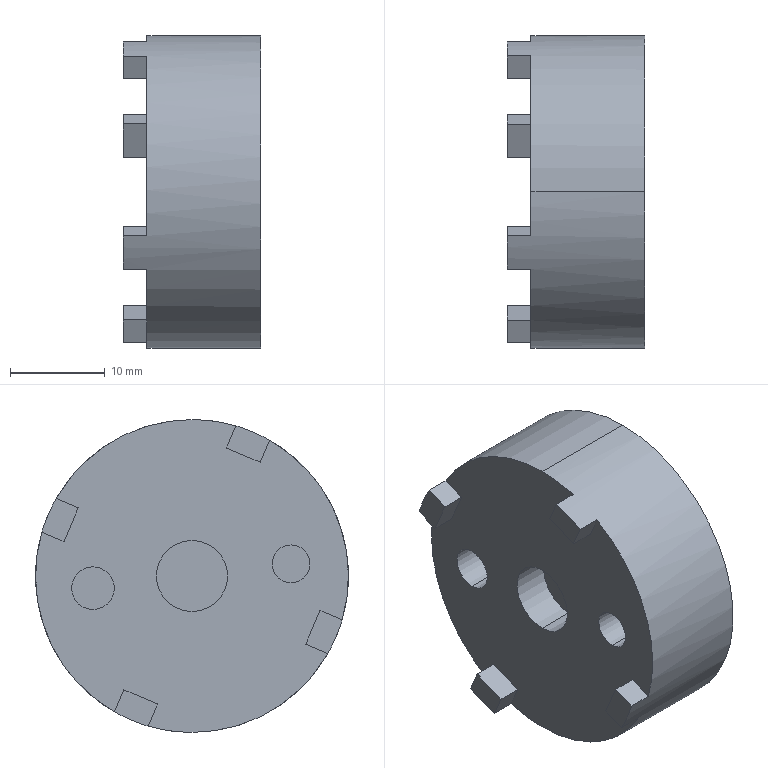Part | SolidWorks | features Cut 2, ICE 2, CirPattern 1, Extrusion 1 | 1 solid | 34 faces | box 14.5 x 33 x 33 mm | volume 10024 mm3 | plane 26 | cylinder 8 | commonest cylinder face diameters 4 x2 4.5 x2 7.5 x2 33 x2
STEP:
#1=CARTESIAN_POINT('',(4.,-10.447,3.283));
#2=VERTEX_POINT('',#1);
#3=CARTESIAN_POINT('',(4.,-10.447,-0.7173));
#4=VERTEX_POINT('',#3);
#5=CARTESIAN_POINT('',(4.,-10.447,1.283));
#6=DIRECTION('',(1.,0.,0.));
#7=DIRECTION('',(0.,0.,1.));
#8=AXIS2_PLACEMENT_3D('',#5,#6,#7);
#9=CIRCLE('',#8,2.);
#10=EDGE_CURVE('',#2,#4,#9,.T.);
#11=ORIENTED_EDGE('',*,*,#10,.T.);
#12=CARTESIAN_POINT('',(0.,-10.447,-0.7173));
#13=VERTEX_POINT('',#12);
#14=CARTESIAN_POINT('',(10.364,-10.447,-0.7173));
#15=DIRECTION('',(-1.,0.,0.));
#16=VECTOR('',#15,1000.);
#17=LINE('',#14,#16);
#18=EDGE_CURVE('',#4,#13,#17,.T.);
#19=ORIENTED_EDGE('',*,*,#18,.T.);
#20=CARTESIAN_POINT('',(0.,-10.447,3.283));
#21=VERTEX_POINT('',#20);
#22=CARTESIAN_POINT('',(0.,-10.447,1.283));
#23=DIRECTION('',(-1.,0.,0.));
#24=DIRECTION('',(0.,0.,1.));
#25=AXIS2_PLACEMENT_3D('',#22,#23,#24);
#26=CIRCLE('',#25,2.);
#27=EDGE_CURVE('',#13,#21,#26,.T.);
#28=ORIENTED_EDGE('',*,*,#27,.T.);
#29=CARTESIAN_POINT('',(10.364,-10.447,3.283));
#30=DIRECTION('',(-1.,0.,0.));
#31=VECTOR('',#30,1000.);
#32=LINE('',#29,#31);
#33=EDGE_CURVE('',#2,#21,#32,.T.);
#34=ORIENTED_EDGE('',*,*,#33,.F.);
#35=EDGE_LOOP('',(#11,#19,#28,#34));
#36=FACE_OUTER_BOUND('',#35,.T.);
#37=CARTESIAN_POINT('',(10.364,-10.447,1.283));
#38=DIRECTION('',(-1.,0.,0.));
#39=DIRECTION('',(0.,0.,1.));
#40=AXIS2_PLACEMENT_3D('',#37,#38,#39);
#41=CYLINDRICAL_SURFACE('',#40,2.);
#42=ADVANCED_FACE('',(#36),#41,.F.);
#43=CARTESIAN_POINT('',(4.,10.447,0.9673));
#44=VERTEX_POINT('',#43);
#45=CARTESIAN_POINT('',(4.,10.447,-3.533));
#46=VERTEX_POINT('',#45);
#47=CARTESIAN_POINT('',(4.,10.447,-1.283));
#48=DIRECTION('',(1.,0.,0.));
#49=DIRECTION('',(0.,0.,1.));
#50=AXIS2_PLACEMENT_3D('',#47,#48,#49);
#51=CIRCLE('',#50,2.25);
#52=EDGE_CURVE('',#44,#46,#51,.T.);
#53=ORIENTED_EDGE('',*,*,#52,.T.);
#54=CARTESIAN_POINT('',(0.,10.447,-3.533));
#55=VERTEX_POINT('',#54);
#56=CARTESIAN_POINT('',(10.364,10.447,-3.533));
#57=DIRECTION('',(-1.,0.,0.));
#58=VECTOR('',#57,1000.);
#59=LINE('',#56,#58);
#60=EDGE_CURVE('',#46,#55,#59,.T.);
#61=ORIENTED_EDGE('',*,*,#60,.T.);
#62=CARTESIAN_POINT('',(0.,10.447,0.9673));
#63=VERTEX_POINT('',#62);
#64=CARTESIAN_POINT('',(0.,10.447,-1.283));
#65=DIRECTION('',(-1.,0.,0.));
#66=DIRECTION('',(0.,0.,1.));
#67=AXIS2_PLACEMENT_3D('',#64,#65,#66);
#68=CIRCLE('',#67,2.25);
#69=EDGE_CURVE('',#55,#63,#68,.T.);
#70=ORIENTED_EDGE('',*,*,#69,.T.);
#71=CARTESIAN_POINT('',(10.364,10.447,0.9673));
#72=DIRECTION('',(-1.,0.,0.));
#73=VECTOR('',#72,1000.);
#74=LINE('',#71,#73);
#75=EDGE_CURVE('',#44,#63,#74,.T.);
#76=ORIENTED_EDGE('',*,*,#75,.F.);
#77=EDGE_LOOP('',(#53,#61,#70,#76));
#78=FACE_OUTER_BOUND('',#77,.T.);
#79=CARTESIAN_POINT('',(10.364,10.447,-1.283));
#80=DIRECTION('',(-1.,0.,0.));
#81=DIRECTION('',(0.,0.,1.));
#82=AXIS2_PLACEMENT_3D('',#79,#80,#81);
#83=CYLINDRICAL_SURFACE('',#82,2.25);
#84=ADVANCED_FACE('',(#78),#83,.F.);
#85=CARTESIAN_POINT('',(4.,0.,-3.75));
#86=VERTEX_POINT('',#85);
#87=CARTESIAN_POINT('',(4.,0.,3.75));
#88=VERTEX_POINT('',#87);
#89=CARTESIAN_POINT('',(4.,0.,0.));
#90=DIRECTION('',(-1.,0.,0.));
#91=DIRECTION('',(0.,0.,1.));
#92=AXIS2_PLACEMENT_3D('',#89,#90,#91);
#93=CIRCLE('',#92,3.75);
#94=EDGE_CURVE('',#86,#88,#93,.T.);
#95=ORIENTED_EDGE('',*,*,#94,.F.);
#96=CARTESIAN_POINT('',(0.,0.,-3.75));
#97=VERTEX_POINT('',#96);
#98=CARTESIAN_POINT('',(4.,0.,-3.75));
#99=DIRECTION('',(-1.,0.,0.));
#100=VECTOR('',#99,1000.);
#101=LINE('',#98,#100);
#102=EDGE_CURVE('',#86,#97,#101,.T.);
#103=ORIENTED_EDGE('',*,*,#102,.T.);
#104=CARTESIAN_POINT('',(0.,0.,3.75));
#105=VERTEX_POINT('',#104);
#106=CARTESIAN_POINT('',(0.,0.,0.));
#107=DIRECTION('',(-1.,0.,0.));
#108=DIRECTION('',(0.,0.,1.));
#109=AXIS2_PLACEMENT_3D('',#106,#107,#108);
#110=CIRCLE('',#109,3.75);
#111=EDGE_CURVE('',#97,#105,#110,.T.);
#112=ORIENTED_EDGE('',*,*,#111,.T.);
#113=CARTESIAN_POINT('',(4.,0.,3.75));
#114=DIRECTION('',(-1.,0.,0.));
#115=VECTOR('',#114,1000.);
#116=LINE('',#113,#115);
#117=EDGE_CURVE('',#88,#105,#116,.T.);
#118=ORIENTED_EDGE('',*,*,#117,.F.);
#119=EDGE_LOOP('',(#95,#103,#112,#118));
#120=FACE_OUTER_BOUND('',#119,.T.);
#121=CARTESIAN_POINT('',(4.,0.,0.));
#122=DIRECTION('',(-1.,0.,0.));
#123=DIRECTION('',(0.,0.,1.));
#124=AXIS2_PLACEMENT_3D('',#121,#122,#123);
#125=CYLINDRICAL_SURFACE('',#124,3.75);
#126=ADVANCED_FACE('',(#120),#125,.F.);
#127=CARTESIAN_POINT('',(12.,0.,-16.5));
#128=VERTEX_POINT('',#127);
#129=CARTESIAN_POINT('',(12.,0.,16.5));
#130=VERTEX_POINT('',#129);
#131=CARTESIAN_POINT('',(12.,0.,0.));
#132=DIRECTION('',(1.,0.,0.));
#133=DIRECTION('',(0.,0.,-1.));
#134=AXIS2_PLACEMENT_3D('',#131,#132,#133);
#135=CIRCLE('',#134,16.5);
#136=EDGE_CURVE('',#128,#130,#135,.T.);
#137=ORIENTED_EDGE('',*,*,#136,.F.);
#138=CARTESIAN_POINT('',(0.,0.,-16.5));
#139=VERTEX_POINT('',#138);
#140=CARTESIAN_POINT('',(12.,0.,-16.5));
#141=DIRECTION('',(-1.,0.,0.));
#142=VECTOR('',#141,1000.);
#143=LINE('',#140,#142);
#144=EDGE_CURVE('',#128,#139,#143,.T.);
#145=ORIENTED_EDGE('',*,*,#144,.T.);
#146=CARTESIAN_POINT('',(0.,4.631,-15.837));
#147=VERTEX_POINT('',#146);
#148=CARTESIAN_POINT('',(0.,0.,0.));
#149=DIRECTION('',(1.,0.,0.));
#150=DIRECTION('',(0.,0.,-1.));
#151=AXIS2_PLACEMENT_3D('',#148,#149,#150);
#152=CIRCLE('',#151,16.5);
#153=EDGE_CURVE('',#139,#147,#152,.T.);
#154=ORIENTED_EDGE('',*,*,#153,.T.);
#155=CARTESIAN_POINT('',(-2.5,4.631,-15.837));
#156=VERTEX_POINT('',#155);
#157=CARTESIAN_POINT('',(-2.5,4.631,-15.837));
#158=DIRECTION('',(1.,0.,0.));
#159=VECTOR('',#158,1000.);
#160=LINE('',#157,#159);
#161=EDGE_CURVE('',#156,#147,#160,.T.);
#162=ORIENTED_EDGE('',*,*,#161,.F.);
#163=CARTESIAN_POINT('',(-2.5,8.175,-14.332));
#164=VERTEX_POINT('',#163);
#165=CARTESIAN_POINT('',(-2.5,0.,0.));
#166=DIRECTION('',(-1.,0.,0.));
#167=DIRECTION('',(0.,-1.,0.));
#168=AXIS2_PLACEMENT_3D('',#165,#166,#167);
#169=CIRCLE('',#168,16.5);
#170=EDGE_CURVE('',#164,#156,#169,.T.);
#171=ORIENTED_EDGE('',*,*,#170,.F.);
#172=CARTESIAN_POINT('',(0.,8.175,-14.332));
#173=VERTEX_POINT('',#172);
#174=CARTESIAN_POINT('',(-2.5,8.175,-14.332));
#175=DIRECTION('',(1.,0.,0.));
#176=VECTOR('',#175,1000.);
#177=LINE('',#174,#176);
#178=EDGE_CURVE('',#164,#173,#177,.T.);
#179=ORIENTED_EDGE('',*,*,#178,.T.);
#180=CARTESIAN_POINT('',(0.,15.837,4.631));
#181=VERTEX_POINT('',#180);
#182=CARTESIAN_POINT('',(0.,0.,0.));
#183=DIRECTION('',(1.,0.,0.));
#184=DIRECTION('',(0.,0.,-1.));
#185=AXIS2_PLACEMENT_3D('',#182,#183,#184);
#186=CIRCLE('',#185,16.5);
#187=EDGE_CURVE('',#173,#181,#186,.T.);
#188=ORIENTED_EDGE('',*,*,#187,.T.);
#189=CARTESIAN_POINT('',(-2.5,15.837,4.631));
#190=VERTEX_POINT('',#189);
#191=CARTESIAN_POINT('',(-2.5,15.837,4.631));
#192=DIRECTION('',(1.,0.,0.));
#193=VECTOR('',#192,1000.);
#194=LINE('',#191,#193);
#195=EDGE_CURVE('',#190,#181,#194,.T.);
#196=ORIENTED_EDGE('',*,*,#195,.F.);
#197=CARTESIAN_POINT('',(-2.5,14.332,8.175));
#198=VERTEX_POINT('',#197);
#199=CARTESIAN_POINT('',(-2.5,0.,0.));
#200=DIRECTION('',(-1.,0.,0.));
#201=DIRECTION('',(0.,0.,-1.));
#202=AXIS2_PLACEMENT_3D('',#199,#200,#201);
#203=CIRCLE('',#202,16.5);
#204=EDGE_CURVE('',#198,#190,#203,.T.);
#205=ORIENTED_EDGE('',*,*,#204,.F.);
#206=CARTESIAN_POINT('',(0.,14.332,8.175));
#207=VERTEX_POINT('',#206);
#208=CARTESIAN_POINT('',(-2.5,14.332,8.175));
#209=DIRECTION('',(1.,0.,0.));
#210=VECTOR('',#209,1000.);
#211=LINE('',#208,#210);
#212=EDGE_CURVE('',#198,#207,#211,.T.);
#213=ORIENTED_EDGE('',*,*,#212,.T.);
#214=CARTESIAN_POINT('',(0.,0.,16.5));
#215=VERTEX_POINT('',#214);
#216=CARTESIAN_POINT('',(0.,0.,0.));
#217=DIRECTION('',(1.,0.,0.));
#218=DIRECTION('',(0.,0.,-1.));
#219=AXIS2_PLACEMENT_3D('',#216,#217,#218);
#220=CIRCLE('',#219,16.5);
#221=EDGE_CURVE('',#207,#215,#220,.T.);
#222=ORIENTED_EDGE('',*,*,#221,.T.);
#223=CARTESIAN_POINT('',(12.,0.,16.5));
#224=DIRECTION('',(-1.,0.,0.));
#225=VECTOR('',#224,1000.);
#226=LINE('',#223,#225);
#227=EDGE_CURVE('',#130,#215,#226,.T.);
#228=ORIENTED_EDGE('',*,*,#227,.F.);
#229=EDGE_LOOP('',(#137,#145,#154,#162,#171,#179,#188,#196,#205,#213,#222,#228));
#230=FACE_OUTER_BOUND('',#229,.T.);
#231=CARTESIAN_POINT('',(12.,0.,0.));
#232=DIRECTION('',(-1.,0.,0.));
#233=DIRECTION('',(0.,0.,1.));
#234=AXIS2_PLACEMENT_3D('',#231,#232,#233);
#235=CYLINDRICAL_SURFACE('',#234,16.5);
#236=ADVANCED_FACE('',(#230),#235,.T.);
#237=CARTESIAN_POINT('',(0.,3.64,-13.501));
#238=VERTEX_POINT('',#237);
#239=CARTESIAN_POINT('',(0.,7.184,-11.997));
#240=VERTEX_POINT('',#239);
#241=CARTESIAN_POINT('',(0.,3.64,-13.501));
#242=DIRECTION('',(0.,0.9205,0.3907));
#243=VECTOR('',#242,1000.);
#244=LINE('',#241,#243);
#245=EDGE_CURVE('',#238,#240,#244,.T.);
#246=ORIENTED_EDGE('',*,*,#245,.T.);
#247=CARTESIAN_POINT('',(-2.5,7.184,-11.997));
#248=VERTEX_POINT('',#247);
#249=CARTESIAN_POINT('',(-2.5,7.184,-11.997));
#250=DIRECTION('',(1.,0.,0.));
#251=VECTOR('',#250,1000.);
#252=LINE('',#249,#251);
#253=EDGE_CURVE('',#248,#240,#252,.T.);
#254=ORIENTED_EDGE('',*,*,#253,.F.);
#255=CARTESIAN_POINT('',(-2.5,3.64,-13.501));
#256=VERTEX_POINT('',#255);
#257=CARTESIAN_POINT('',(-2.5,3.64,-13.501));
#258=DIRECTION('',(0.,0.9205,0.3907));
#259=VECTOR('',#258,1000.);
#260=LINE('',#257,#259);
#261=EDGE_CURVE('',#256,#248,#260,.T.);
#262=ORIENTED_EDGE('',*,*,#261,.F.);
#263=CARTESIAN_POINT('',(-2.5,3.64,-13.501));
#264=DIRECTION('',(1.,0.,0.));
#265=VECTOR('',#264,1000.);
#266=LINE('',#263,#265);
#267=EDGE_CURVE('',#256,#238,#266,.T.);
#268=ORIENTED_EDGE('',*,*,#267,.T.);
#269=EDGE_LOOP('',(#246,#254,#262,#268));
#270=FACE_OUTER_BOUND('',#269,.T.);
#271=CARTESIAN_POINT('',(-2.5,3.64,-13.501));
#272=DIRECTION('',(0.,0.3907,-0.9205));
#273=DIRECTION('',(0.,0.9205,0.3907));
#274=AXIS2_PLACEMENT_3D('',#271,#272,#273);
#275=PLANE('',#274);
#276=ADVANCED_FACE('',(#270),#275,.F.);
#277=CARTESIAN_POINT('',(0.,7.184,-11.997));
#278=DIRECTION('',(0.,0.3907,-0.9205));
#279=VECTOR('',#278,1000.);
#280=LINE('',#277,#279);
#281=EDGE_CURVE('',#240,#173,#280,.T.);
#282=ORIENTED_EDGE('',*,*,#281,.T.);
#283=ORIENTED_EDGE('',*,*,#178,.F.);
#284=CARTESIAN_POINT('',(-2.5,7.184,-11.997));
#285=DIRECTION('',(0.,0.3907,-0.9205));
#286=VECTOR('',#285,1000.);
#287=LINE('',#284,#286);
#288=EDGE_CURVE('',#248,#164,#287,.T.);
#289=ORIENTED_EDGE('',*,*,#288,.F.);
#290=ORIENTED_EDGE('',*,*,#253,.T.);
#291=EDGE_LOOP('',(#282,#283,#289,#290));
#292=FACE_OUTER_BOUND('',#291,.T.);
#293=CARTESIAN_POINT('',(-2.5,7.184,-11.997));
#294=DIRECTION('',(0.,-0.9205,-0.3907));
#295=DIRECTION('',(0.,0.3907,-0.9205));
#296=AXIS2_PLACEMENT_3D('',#293,#294,#295);
#297=PLANE('',#296);
#298=ADVANCED_FACE('',(#292),#297,.F.);
#299=CARTESIAN_POINT('',(0.,3.64,-13.501));
#300=DIRECTION('',(0.,-0.3907,0.9205));
#301=VECTOR('',#300,1000.);
#302=LINE('',#299,#301);
#303=EDGE_CURVE('',#147,#238,#302,.T.);
#304=ORIENTED_EDGE('',*,*,#303,.T.);
#305=ORIENTED_EDGE('',*,*,#267,.F.);
#306=CARTESIAN_POINT('',(-2.5,3.64,-13.501));
#307=DIRECTION('',(0.,-0.3907,0.9205));
#308=VECTOR('',#307,1000.);
#309=LINE('',#306,#308);
#310=EDGE_CURVE('',#156,#256,#309,.T.);
#311=ORIENTED_EDGE('',*,*,#310,.F.);
#312=ORIENTED_EDGE('',*,*,#161,.T.);
#313=EDGE_LOOP('',(#304,#305,#311,#312));
#314=FACE_OUTER_BOUND('',#313,.T.);
#315=CARTESIAN_POINT('',(-2.5,3.64,-13.501));
#316=DIRECTION('',(0.,0.9205,0.3907));
#317=DIRECTION('',(0.,-0.3907,0.9205));
#318=AXIS2_PLACEMENT_3D('',#315,#316,#317);
#319=PLANE('',#318);
#320=ADVANCED_FACE('',(#314),#319,.F.);
#321=ORIENTED_EDGE('',*,*,#261,.T.);
#322=ORIENTED_EDGE('',*,*,#288,.T.);
#323=ORIENTED_EDGE('',*,*,#170,.T.);
#324=ORIENTED_EDGE('',*,*,#310,.T.);
#325=EDGE_LOOP('',(#321,#322,#323,#324));
#326=FACE_OUTER_BOUND('',#325,.T.);
#327=CARTESIAN_POINT('',(-2.5,0.,0.));
#328=DIRECTION('',(-1.,0.,0.));
#329=DIRECTION('',(0.,-1.,0.));
#330=AXIS2_PLACEMENT_3D('',#327,#328,#329);
#331=PLANE('',#330);
#332=ADVANCED_FACE('',(#326),#331,.T.);
#333=CARTESIAN_POINT('',(0.,13.501,3.64));
#334=VERTEX_POINT('',#333);
#335=CARTESIAN_POINT('',(0.,11.997,7.184));
#336=VERTEX_POINT('',#335);
#337=CARTESIAN_POINT('',(0.,13.501,3.64));
#338=DIRECTION('',(0.,-0.3907,0.9205));
#339=VECTOR('',#338,1000.);
#340=LINE('',#337,#339);
#341=EDGE_CURVE('',#334,#336,#340,.T.);
#342=ORIENTED_EDGE('',*,*,#341,.T.);
#343=CARTESIAN_POINT('',(-2.5,11.997,7.184));
#344=VERTEX_POINT('',#343);
#345=CARTESIAN_POINT('',(-2.5,11.997,7.184));
#346=DIRECTION('',(1.,0.,0.));
#347=VECTOR('',#346,1000.);
#348=LINE('',#345,#347);
#349=EDGE_CURVE('',#344,#336,#348,.T.);
#350=ORIENTED_EDGE('',*,*,#349,.F.);
#351=CARTESIAN_POINT('',(-2.5,13.501,3.64));
#352=VERTEX_POINT('',#351);
#353=CARTESIAN_POINT('',(-2.5,13.501,3.64));
#354=DIRECTION('',(0.,-0.3907,0.9205));
#355=VECTOR('',#354,1000.);
#356=LINE('',#353,#355);
#357=EDGE_CURVE('',#352,#344,#356,.T.);
#358=ORIENTED_EDGE('',*,*,#357,.F.);
#359=CARTESIAN_POINT('',(-2.5,13.501,3.64));
#360=DIRECTION('',(1.,0.,0.));
#361=VECTOR('',#360,1000.);
#362=LINE('',#359,#361);
#363=EDGE_CURVE('',#352,#334,#362,.T.);
#364=ORIENTED_EDGE('',*,*,#363,.T.);
#365=EDGE_LOOP('',(#342,#350,#358,#364));
#366=FACE_OUTER_BOUND('',#365,.T.);
#367=CARTESIAN_POINT('',(-2.5,13.501,3.64));
#368=DIRECTION('',(0.,0.9205,0.3907));
#369=DIRECTION('',(0.,-0.3907,0.9205));
#370=AXIS2_PLACEMENT_3D('',#367,#368,#369);
#371=PLANE('',#370);
#372=ADVANCED_FACE('',(#366),#371,.F.);
#373=CARTESIAN_POINT('',(0.,11.997,7.184));
#374=DIRECTION('',(0.,0.9205,0.3907));
#375=VECTOR('',#374,1000.);
#376=LINE('',#373,#375);
#377=EDGE_CURVE('',#336,#207,#376,.T.);
#378=ORIENTED_EDGE('',*,*,#377,.T.);
#379=ORIENTED_EDGE('',*,*,#212,.F.);
#380=CARTESIAN_POINT('',(-2.5,11.997,7.184));
#381=DIRECTION('',(0.,0.9205,0.3907));
#382=VECTOR('',#381,1000.);
#383=LINE('',#380,#382);
#384=EDGE_CURVE('',#344,#198,#383,.T.);
#385=ORIENTED_EDGE('',*,*,#384,.F.);
#386=ORIENTED_EDGE('',*,*,#349,.T.);
#387=EDGE_LOOP('',(#378,#379,#385,#386));
#388=FACE_OUTER_BOUND('',#387,.T.);
#389=CARTESIAN_POINT('',(-2.5,11.997,7.184));
#390=DIRECTION('',(0.,0.3907,-0.9205));
#391=DIRECTION('',(0.,0.9205,0.3907));
#392=AXIS2_PLACEMENT_3D('',#389,#390,#391);
#393=PLANE('',#392);
#394=ADVANCED_FACE('',(#388),#393,.F.);
#395=CARTESIAN_POINT('',(0.,13.501,3.64));
#396=DIRECTION('',(0.,-0.9205,-0.3907));
#397=VECTOR('',#396,1000.);
#398=LINE('',#395,#397);
#399=EDGE_CURVE('',#181,#334,#398,.T.);
#400=ORIENTED_EDGE('',*,*,#399,.T.);
#401=ORIENTED_EDGE('',*,*,#363,.F.);
#402=CARTESIAN_POINT('',(-2.5,13.501,3.64));
#403=DIRECTION('',(0.,-0.9205,-0.3907));
#404=VECTOR('',#403,1000.);
#405=LINE('',#402,#404);
#406=EDGE_CURVE('',#190,#352,#405,.T.);
#407=ORIENTED_EDGE('',*,*,#406,.F.);
#408=ORIENTED_EDGE('',*,*,#195,.T.);
#409=EDGE_LOOP('',(#400,#401,#407,#408));
#410=FACE_OUTER_BOUND('',#409,.T.);
#411=CARTESIAN_POINT('',(-2.5,13.501,3.64));
#412=DIRECTION('',(0.,-0.3907,0.9205));
#413=DIRECTION('',(0.,-0.9205,-0.3907));
#414=AXIS2_PLACEMENT_3D('',#411,#412,#413);
#415=PLANE('',#414);
#416=ADVANCED_FACE('',(#410),#415,.F.);
#417=ORIENTED_EDGE('',*,*,#357,.T.);
#418=ORIENTED_EDGE('',*,*,#384,.T.);
#419=ORIENTED_EDGE('',*,*,#204,.T.);
#420=ORIENTED_EDGE('',*,*,#406,.T.);
#421=EDGE_LOOP('',(#417,#418,#419,#420));
#422=FACE_OUTER_BOUND('',#421,.T.);
#423=CARTESIAN_POINT('',(-2.5,0.,0.));
#424=DIRECTION('',(-1.,0.,0.));
#425=DIRECTION('',(0.,0.,-1.));
#426=AXIS2_PLACEMENT_3D('',#423,#424,#425);
#427=PLANE('',#426);
#428=ADVANCED_FACE('',(#422),#427,.T.);
#429=CARTESIAN_POINT('',(0.,-3.64,13.501));
#430=VERTEX_POINT('',#429);
#431=CARTESIAN_POINT('',(0.,-7.184,11.997));
#432=VERTEX_POINT('',#431);
#433=CARTESIAN_POINT('',(0.,-3.64,13.501));
#434=DIRECTION('',(0.,-0.9205,-0.3907));
#435=VECTOR('',#434,1000.);
#436=LINE('',#433,#435);
#437=EDGE_CURVE('',#430,#432,#436,.T.);
#438=ORIENTED_EDGE('',*,*,#437,.T.);
#439=CARTESIAN_POINT('',(-2.5,-7.184,11.997));
#440=VERTEX_POINT('',#439);
#441=CARTESIAN_POINT('',(-2.5,-7.184,11.997));
#442=DIRECTION('',(1.,0.,0.));
#443=VECTOR('',#442,1000.);
#444=LINE('',#441,#443);
#445=EDGE_CURVE('',#440,#432,#444,.T.);
#446=ORIENTED_EDGE('',*,*,#445,.F.);
#447=CARTESIAN_POINT('',(-2.5,-3.64,13.501));
#448=VERTEX_POINT('',#447);
#449=CARTESIAN_POINT('',(-2.5,-3.64,13.501));
#450=DIRECTION('',(0.,-0.9205,-0.3907));
#451=VECTOR('',#450,1000.);
#452=LINE('',#449,#451);
#453=EDGE_CURVE('',#448,#440,#452,.T.);
#454=ORIENTED_EDGE('',*,*,#453,.F.);
#455=CARTESIAN_POINT('',(-2.5,-3.64,13.501));
#456=DIRECTION('',(1.,0.,0.));
#457=VECTOR('',#456,1000.);
#458=LINE('',#455,#457);
#459=EDGE_CURVE('',#448,#430,#458,.T.);
#460=ORIENTED_EDGE('',*,*,#459,.T.);
#461=EDGE_LOOP('',(#438,#446,#454,#460));
#462=FACE_OUTER_BOUND('',#461,.T.);
#463=CARTESIAN_POINT('',(-2.5,-3.64,13.501));
#464=DIRECTION('',(0.,-0.3907,0.9205));
#465=DIRECTION('',(0.,-0.9205,-0.3907));
#466=AXIS2_PLACEMENT_3D('',#463,#464,#465);
#467=PLANE('',#466);
#468=ADVANCED_FACE('',(#462),#467,.F.);
#469=CARTESIAN_POINT('',(0.,-8.175,14.332));
#470=VERTEX_POINT('',#469);
#471=CARTESIAN_POINT('',(0.,-7.184,11.997));
#472=DIRECTION('',(0.,-0.3907,0.9205));
#473=VECTOR('',#472,1000.);
#474=LINE('',#471,#473);
#475=EDGE_CURVE('',#432,#470,#474,.T.);
#476=ORIENTED_EDGE('',*,*,#475,.T.);
#477=CARTESIAN_POINT('',(-2.5,-8.175,14.332));
#478=VERTEX_POINT('',#477);
#479=CARTESIAN_POINT('',(-2.5,-8.175,14.332));
#480=DIRECTION('',(1.,0.,0.));
#481=VECTOR('',#480,1000.);
#482=LINE('',#479,#481);
#483=EDGE_CURVE('',#478,#470,#482,.T.);
#484=ORIENTED_EDGE('',*,*,#483,.F.);
#485=CARTESIAN_POINT('',(-2.5,-7.184,11.997));
#486=DIRECTION('',(0.,-0.3907,0.9205));
#487=VECTOR('',#486,1000.);
#488=LINE('',#485,#487);
#489=EDGE_CURVE('',#440,#478,#488,.T.);
#490=ORIENTED_EDGE('',*,*,#489,.F.);
#491=ORIENTED_EDGE('',*,*,#445,.T.);
#492=EDGE_LOOP('',(#476,#484,#490,#491));
#493=FACE_OUTER_BOUND('',#492,.T.);
#494=CARTESIAN_POINT('',(-2.5,-7.184,11.997));
#495=DIRECTION('',(0.,0.9205,0.3907));
#496=DIRECTION('',(0.,-0.3907,0.9205));
#497=AXIS2_PLACEMENT_3D('',#494,#495,#496);
#498=PLANE('',#497);
#499=ADVANCED_FACE('',(#493),#498,.F.);
#500=CARTESIAN_POINT('',(0.,-4.631,15.837));
#501=VERTEX_POINT('',#500);
#502=CARTESIAN_POINT('',(0.,-3.64,13.501));
#503=DIRECTION('',(0.,0.3907,-0.9205));
#504=VECTOR('',#503,1000.);
#505=LINE('',#502,#504);
#506=EDGE_CURVE('',#501,#430,#505,.T.);
#507=ORIENTED_EDGE('',*,*,#506,.T.);
#508=ORIENTED_EDGE('',*,*,#459,.F.);
#509=CARTESIAN_POINT('',(-2.5,-4.631,15.837));
#510=VERTEX_POINT('',#509);
#511=CARTESIAN_POINT('',(-2.5,-3.64,13.501));
#512=DIRECTION('',(0.,0.3907,-0.9205));
#513=VECTOR('',#512,1000.);
#514=LINE('',#511,#513);
#515=EDGE_CURVE('',#510,#448,#514,.T.);
#516=ORIENTED_EDGE('',*,*,#515,.F.);
#517=CARTESIAN_POINT('',(-2.5,-4.631,15.837));
#518=DIRECTION('',(1.,0.,0.));
#519=VECTOR('',#518,1000.);
#520=LINE('',#517,#519);
#521=EDGE_CURVE('',#510,#501,#520,.T.);
#522=ORIENTED_EDGE('',*,*,#521,.T.);
#523=EDGE_LOOP('',(#507,#508,#516,#522));
#524=FACE_OUTER_BOUND('',#523,.T.);
#525=CARTESIAN_POINT('',(-2.5,-3.64,13.501));
#526=DIRECTION('',(0.,-0.9205,-0.3907));
#527=DIRECTION('',(0.,0.3907,-0.9205));
#528=AXIS2_PLACEMENT_3D('',#525,#526,#527);
#529=PLANE('',#528);
#530=ADVANCED_FACE('',(#524),#529,.F.);
#531=ORIENTED_EDGE('',*,*,#453,.T.);
#532=ORIENTED_EDGE('',*,*,#489,.T.);
#533=CARTESIAN_POINT('',(-2.5,0.,0.));
#534=DIRECTION('',(-1.,0.,0.));
#535=DIRECTION('',(0.,1.,0.));
#536=AXIS2_PLACEMENT_3D('',#533,#534,#535);
#537=CIRCLE('',#536,16.5);
#538=EDGE_CURVE('',#478,#510,#537,.T.);
#539=ORIENTED_EDGE('',*,*,#538,.T.);
#540=ORIENTED_EDGE('',*,*,#515,.T.);
#541=EDGE_LOOP('',(#531,#532,#539,#540));
#542=FACE_OUTER_BOUND('',#541,.T.);
#543=CARTESIAN_POINT('',(-2.5,0.,0.));
#544=DIRECTION('',(-1.,0.,0.));
#545=DIRECTION('',(0.,1.,0.));
#546=AXIS2_PLACEMENT_3D('',#543,#544,#545);
#547=PLANE('',#546);
#548=ADVANCED_FACE('',(#542),#547,.T.);
#549=CARTESIAN_POINT('',(0.,-10.447,1.283));
#550=DIRECTION('',(-1.,0.,0.));
#551=DIRECTION('',(0.,0.,1.));
#552=AXIS2_PLACEMENT_3D('',#549,#550,#551);
#553=CIRCLE('',#552,2.);
#554=EDGE_CURVE('',#21,#13,#553,.T.);
#555=ORIENTED_EDGE('',*,*,#554,.F.);
#556=ORIENTED_EDGE('',*,*,#27,.F.);
#557=EDGE_LOOP('',(#555,#556));
#558=FACE_BOUND('',#557,.T.);
#559=CARTESIAN_POINT('',(0.,10.447,-1.283));
#560=DIRECTION('',(-1.,0.,0.));
#561=DIRECTION('',(0.,0.,1.));
#562=AXIS2_PLACEMENT_3D('',#559,#560,#561);
#563=CIRCLE('',#562,2.25);
#564=EDGE_CURVE('',#63,#55,#563,.T.);
#565=ORIENTED_EDGE('',*,*,#564,.F.);
#566=ORIENTED_EDGE('',*,*,#69,.F.);
#567=EDGE_LOOP('',(#565,#566));
#568=FACE_BOUND('',#567,.T.);
#569=CARTESIAN_POINT('',(0.,0.,0.));
#570=DIRECTION('',(-1.,0.,0.));
#571=DIRECTION('',(0.,0.,1.));
#572=AXIS2_PLACEMENT_3D('',#569,#570,#571);
#573=CIRCLE('',#572,3.75);
#574=EDGE_CURVE('',#105,#97,#573,.T.);
#575=ORIENTED_EDGE('',*,*,#574,.F.);
#576=ORIENTED_EDGE('',*,*,#111,.F.);
#577=EDGE_LOOP('',(#575,#576));
#578=FACE_BOUND('',#577,.T.);
#579=CARTESIAN_POINT('',(0.,-14.332,-8.175));
#580=VERTEX_POINT('',#579);
#581=CARTESIAN_POINT('',(0.,0.,0.));
#582=DIRECTION('',(1.,0.,0.));
#583=DIRECTION('',(0.,0.,-1.));
#584=AXIS2_PLACEMENT_3D('',#581,#582,#583);
#585=CIRCLE('',#584,16.5);
#586=EDGE_CURVE('',#580,#139,#585,.T.);
#587=ORIENTED_EDGE('',*,*,#586,.F.);
#588=CARTESIAN_POINT('',(0.,-11.997,-7.184));
#589=VERTEX_POINT('',#588);
#590=CARTESIAN_POINT('',(0.,-11.997,-7.184));
#591=DIRECTION('',(0.,-0.9205,-0.3907));
#592=VECTOR('',#591,1000.);
#593=LINE('',#590,#592);
#594=EDGE_CURVE('',#589,#580,#593,.T.);
#595=ORIENTED_EDGE('',*,*,#594,.F.);
#596=CARTESIAN_POINT('',(0.,-13.501,-3.64));
#597=VERTEX_POINT('',#596);
#598=CARTESIAN_POINT('',(0.,-13.501,-3.64));
#599=DIRECTION('',(0.,0.3907,-0.9205));
#600=VECTOR('',#599,1000.);
#601=LINE('',#598,#600);
#602=EDGE_CURVE('',#597,#589,#601,.T.);
#603=ORIENTED_EDGE('',*,*,#602,.F.);
#604=CARTESIAN_POINT('',(0.,-15.837,-4.631));
#605=VERTEX_POINT('',#604);
#606=CARTESIAN_POINT('',(0.,-13.501,-3.64));
#607=DIRECTION('',(0.,0.9205,0.3907));
#608=VECTOR('',#607,1000.);
#609=LINE('',#606,#608);
#610=EDGE_CURVE('',#605,#597,#609,.T.);
#611=ORIENTED_EDGE('',*,*,#610,.F.);
#612=CARTESIAN_POINT('',(0.,0.,0.));
#613=DIRECTION('',(1.,0.,0.));
#614=DIRECTION('',(0.,0.,-1.));
#615=AXIS2_PLACEMENT_3D('',#612,#613,#614);
#616=CIRCLE('',#615,16.5);
#617=EDGE_CURVE('',#470,#605,#616,.T.);
#618=ORIENTED_EDGE('',*,*,#617,.F.);
#619=ORIENTED_EDGE('',*,*,#475,.F.);
#620=ORIENTED_EDGE('',*,*,#437,.F.);
#621=ORIENTED_EDGE('',*,*,#506,.F.);
#622=CARTESIAN_POINT('',(0.,0.,0.));
#623=DIRECTION('',(1.,0.,0.));
#624=DIRECTION('',(0.,0.,-1.));
#625=AXIS2_PLACEMENT_3D('',#622,#623,#624);
#626=CIRCLE('',#625,16.5);
#627=EDGE_CURVE('',#215,#501,#626,.T.);
#628=ORIENTED_EDGE('',*,*,#627,.F.);
#629=ORIENTED_EDGE('',*,*,#221,.F.);
#630=ORIENTED_EDGE('',*,*,#377,.F.);
#631=ORIENTED_EDGE('',*,*,#341,.F.);
#632=ORIENTED_EDGE('',*,*,#399,.F.);
#633=ORIENTED_EDGE('',*,*,#187,.F.);
#634=ORIENTED_EDGE('',*,*,#281,.F.);
#635=ORIENTED_EDGE('',*,*,#245,.F.);
#636=ORIENTED_EDGE('',*,*,#303,.F.);
#637=ORIENTED_EDGE('',*,*,#153,.F.);
#638=EDGE_LOOP('',(#587,#595,#603,#611,#618,#619,#620,#621,#628,#629,#630,#631,#632,#633,#634,#635,#636,#637));
#639=FACE_OUTER_BOUND('',#638,.T.);
#640=CARTESIAN_POINT('',(0.,0.,0.));
#641=DIRECTION('',(1.,0.,0.));
#642=DIRECTION('',(0.,0.,-1.));
#643=AXIS2_PLACEMENT_3D('',#640,#641,#642);
#644=PLANE('',#643);
#645=ADVANCED_FACE('',(#558,#568,#578,#639),#644,.F.);
#646=ORIENTED_EDGE('',*,*,#144,.F.);
#647=CARTESIAN_POINT('',(12.,0.,0.));
#648=DIRECTION('',(1.,0.,0.));
#649=DIRECTION('',(0.,0.,-1.));
#650=AXIS2_PLACEMENT_3D('',#647,#648,#649);
#651=CIRCLE('',#650,16.5);
#652=EDGE_CURVE('',#130,#128,#651,.T.);
#653=ORIENTED_EDGE('',*,*,#652,.F.);
#654=ORIENTED_EDGE('',*,*,#227,.T.);
#655=ORIENTED_EDGE('',*,*,#627,.T.);
#656=ORIENTED_EDGE('',*,*,#521,.F.);
#657=ORIENTED_EDGE('',*,*,#538,.F.);
#658=ORIENTED_EDGE('',*,*,#483,.T.);
#659=ORIENTED_EDGE('',*,*,#617,.T.);
#660=CARTESIAN_POINT('',(-2.5,-15.837,-4.631));
#661=VERTEX_POINT('',#660);
#662=CARTESIAN_POINT('',(-2.5,-15.837,-4.631));
#663=DIRECTION('',(1.,0.,0.));
#664=VECTOR('',#663,1000.);
#665=LINE('',#662,#664);
#666=EDGE_CURVE('',#661,#605,#665,.T.);
#667=ORIENTED_EDGE('',*,*,#666,.F.);
#668=CARTESIAN_POINT('',(-2.5,-14.332,-8.175));
#669=VERTEX_POINT('',#668);
#670=CARTESIAN_POINT('',(-2.5,0.,0.));
#671=DIRECTION('',(-1.,0.,0.));
#672=DIRECTION('',(0.,0.,1.));
#673=AXIS2_PLACEMENT_3D('',#670,#671,#672);
#674=CIRCLE('',#673,16.5);
#675=EDGE_CURVE('',#669,#661,#674,.T.);
#676=ORIENTED_EDGE('',*,*,#675,.F.);
#677=CARTESIAN_POINT('',(-2.5,-14.332,-8.175));
#678=DIRECTION('',(1.,0.,0.));
#679=VECTOR('',#678,1000.);
#680=LINE('',#677,#679);
#681=EDGE_CURVE('',#669,#580,#680,.T.);
#682=ORIENTED_EDGE('',*,*,#681,.T.);
#683=ORIENTED_EDGE('',*,*,#586,.T.);
#684=EDGE_LOOP('',(#646,#653,#654,#655,#656,#657,#658,#659,#667,#676,#682,#683));
#685=FACE_OUTER_BOUND('',#684,.T.);
#686=CARTESIAN_POINT('',(12.,0.,0.));
#687=DIRECTION('',(-1.,0.,0.));
#688=DIRECTION('',(0.,0.,1.));
#689=AXIS2_PLACEMENT_3D('',#686,#687,#688);
#690=CYLINDRICAL_SURFACE('',#689,16.5);
#691=ADVANCED_FACE('',(#685),#690,.T.);
#692=CARTESIAN_POINT('',(12.,-2.5,-2.5));
#693=VERTEX_POINT('',#692);
#694=CARTESIAN_POINT('',(12.,2.5,-2.5));
#695=VERTEX_POINT('',#694);
#696=CARTESIAN_POINT('',(12.,2.5,-2.5));
#697=DIRECTION('',(0.,1.,0.));
#698=VECTOR('',#697,1000.);
#699=LINE('',#696,#698);
#700=EDGE_CURVE('',#693,#695,#699,.T.);
#701=ORIENTED_EDGE('',*,*,#700,.F.);
#702=CARTESIAN_POINT('',(12.,-2.5,2.5));
#703=VERTEX_POINT('',#702);
#704=CARTESIAN_POINT('',(12.,-2.5,2.5));
#705=DIRECTION('',(0.,0.,-1.));
#706=VECTOR('',#705,1000.);
#707=LINE('',#704,#706);
#708=EDGE_CURVE('',#703,#693,#707,.T.);
#709=ORIENTED_EDGE('',*,*,#708,.F.);
#710=CARTESIAN_POINT('',(12.,2.5,2.5));
#711=VERTEX_POINT('',#710);
#712=CARTESIAN_POINT('',(12.,2.5,2.5));
#713=DIRECTION('',(0.,-1.,0.));
#714=VECTOR('',#713,1000.);
#715=LINE('',#712,#714);
#716=EDGE_CURVE('',#711,#703,#715,.T.);
#717=ORIENTED_EDGE('',*,*,#716,.F.);
#718=CARTESIAN_POINT('',(12.,2.5,2.5));
#719=DIRECTION('',(0.,0.,1.));
#720=VECTOR('',#719,1000.);
#721=LINE('',#718,#720);
#722=EDGE_CURVE('',#695,#711,#721,.T.);
#723=ORIENTED_EDGE('',*,*,#722,.F.);
#724=EDGE_LOOP('',(#701,#709,#717,#723));
#725=FACE_BOUND('',#724,.T.);
#726=ORIENTED_EDGE('',*,*,#652,.T.);
#727=ORIENTED_EDGE('',*,*,#136,.T.);
#728=EDGE_LOOP('',(#726,#727));
#729=FACE_OUTER_BOUND('',#728,.T.);
#730=CARTESIAN_POINT('',(12.,0.,0.));
#731=DIRECTION('',(1.,0.,0.));
#732=DIRECTION('',(0.,0.,-1.));
#733=AXIS2_PLACEMENT_3D('',#730,#731,#732);
#734=PLANE('',#733);
#735=ADVANCED_FACE('',(#725,#729),#734,.T.);
#736=ORIENTED_EDGE('',*,*,#102,.F.);
#737=CARTESIAN_POINT('',(4.,0.,0.));
#738=DIRECTION('',(-1.,0.,0.));
#739=DIRECTION('',(0.,0.,1.));
#740=AXIS2_PLACEMENT_3D('',#737,#738,#739);
#741=CIRCLE('',#740,3.75);
#742=EDGE_CURVE('',#88,#86,#741,.T.);
#743=ORIENTED_EDGE('',*,*,#742,.F.);
#744=ORIENTED_EDGE('',*,*,#117,.T.);
#745=ORIENTED_EDGE('',*,*,#574,.T.);
#746=EDGE_LOOP('',(#736,#743,#744,#745));
#747=FACE_OUTER_BOUND('',#746,.T.);
#748=CARTESIAN_POINT('',(4.,0.,0.));
#749=DIRECTION('',(-1.,0.,0.));
#750=DIRECTION('',(0.,0.,1.));
#751=AXIS2_PLACEMENT_3D('',#748,#749,#750);
#752=CYLINDRICAL_SURFACE('',#751,3.75);
#753=ADVANCED_FACE('',(#747),#752,.F.);
#754=ORIENTED_EDGE('',*,*,#742,.T.);
#755=ORIENTED_EDGE('',*,*,#94,.T.);
#756=EDGE_LOOP('',(#754,#755));
#757=FACE_OUTER_BOUND('',#756,.T.);
#758=CARTESIAN_POINT('',(4.,0.,0.));
#759=DIRECTION('',(-1.,0.,0.));
#760=DIRECTION('',(0.,0.,1.));
#761=AXIS2_PLACEMENT_3D('',#758,#759,#760);
#762=PLANE('',#761);
#763=ADVANCED_FACE('',(#757),#762,.T.);
#764=ORIENTED_EDGE('',*,*,#602,.T.);
#765=CARTESIAN_POINT('',(-2.5,-11.997,-7.184));
#766=VERTEX_POINT('',#765);
#767=CARTESIAN_POINT('',(-2.5,-11.997,-7.184));
#768=DIRECTION('',(1.,0.,0.));
#769=VECTOR('',#768,1000.);
#770=LINE('',#767,#769);
#771=EDGE_CURVE('',#766,#589,#770,.T.);
#772=ORIENTED_EDGE('',*,*,#771,.F.);
#773=CARTESIAN_POINT('',(-2.5,-13.501,-3.64));
#774=VERTEX_POINT('',#773);
#775=CARTESIAN_POINT('',(-2.5,-13.501,-3.64));
#776=DIRECTION('',(0.,0.3907,-0.9205));
#777=VECTOR('',#776,1000.);
#778=LINE('',#775,#777);
#779=EDGE_CURVE('',#774,#766,#778,.T.);
#780=ORIENTED_EDGE('',*,*,#779,.F.);
#781=CARTESIAN_POINT('',(-2.5,-13.501,-3.64));
#782=DIRECTION('',(1.,0.,0.));
#783=VECTOR('',#782,1000.);
#784=LINE('',#781,#783);
#785=EDGE_CURVE('',#774,#597,#784,.T.);
#786=ORIENTED_EDGE('',*,*,#785,.T.);
#787=EDGE_LOOP('',(#764,#772,#780,#786));
#788=FACE_OUTER_BOUND('',#787,.T.);
#789=CARTESIAN_POINT('',(-2.5,-13.501,-3.64));
#790=DIRECTION('',(0.,-0.9205,-0.3907));
#791=DIRECTION('',(0.,0.3907,-0.9205));
#792=AXIS2_PLACEMENT_3D('',#789,#790,#791);
#793=PLANE('',#792);
#794=ADVANCED_FACE('',(#788),#793,.F.);
#795=ORIENTED_EDGE('',*,*,#594,.T.);
#796=ORIENTED_EDGE('',*,*,#681,.F.);
#797=CARTESIAN_POINT('',(-2.5,-11.997,-7.184));
#798=DIRECTION('',(0.,-0.9205,-0.3907));
#799=VECTOR('',#798,1000.);
#800=LINE('',#797,#799);
#801=EDGE_CURVE('',#766,#669,#800,.T.);
#802=ORIENTED_EDGE('',*,*,#801,.F.);
#803=ORIENTED_EDGE('',*,*,#771,.T.);
#804=EDGE_LOOP('',(#795,#796,#802,#803));
#805=FACE_OUTER_BOUND('',#804,.T.);
#806=CARTESIAN_POINT('',(-2.5,-11.997,-7.184));
#807=DIRECTION('',(0.,-0.3907,0.9205));
#808=DIRECTION('',(0.,-0.9205,-0.3907));
#809=AXIS2_PLACEMENT_3D('',#806,#807,#808);
#810=PLANE('',#809);
#811=ADVANCED_FACE('',(#805),#810,.F.);
#812=ORIENTED_EDGE('',*,*,#610,.T.);
#813=ORIENTED_EDGE('',*,*,#785,.F.);
#814=CARTESIAN_POINT('',(-2.5,-13.501,-3.64));
#815=DIRECTION('',(0.,0.9205,0.3907));
#816=VECTOR('',#815,1000.);
#817=LINE('',#814,#816);
#818=EDGE_CURVE('',#661,#774,#817,.T.);
#819=ORIENTED_EDGE('',*,*,#818,.F.);
#820=ORIENTED_EDGE('',*,*,#666,.T.);
#821=EDGE_LOOP('',(#812,#813,#819,#820));
#822=FACE_OUTER_BOUND('',#821,.T.);
#823=CARTESIAN_POINT('',(-2.5,-13.501,-3.64));
#824=DIRECTION('',(0.,0.3907,-0.9205));
#825=DIRECTION('',(0.,0.9205,0.3907));
#826=AXIS2_PLACEMENT_3D('',#823,#824,#825);
#827=PLANE('',#826);
#828=ADVANCED_FACE('',(#822),#827,.F.);
#829=ORIENTED_EDGE('',*,*,#779,.T.);
#830=ORIENTED_EDGE('',*,*,#801,.T.);
#831=ORIENTED_EDGE('',*,*,#675,.T.);
#832=ORIENTED_EDGE('',*,*,#818,.T.);
#833=EDGE_LOOP('',(#829,#830,#831,#832));
#834=FACE_OUTER_BOUND('',#833,.T.);
#835=CARTESIAN_POINT('',(-2.5,0.,0.));
#836=DIRECTION('',(-1.,0.,0.));
#837=DIRECTION('',(0.,0.,1.));
#838=AXIS2_PLACEMENT_3D('',#835,#836,#837);
#839=PLANE('',#838);
#840=ADVANCED_FACE('',(#834),#839,.T.);
#841=ORIENTED_EDGE('',*,*,#60,.F.);
#842=CARTESIAN_POINT('',(4.,10.447,-1.283));
#843=DIRECTION('',(1.,0.,0.));
#844=DIRECTION('',(0.,0.,1.));
#845=AXIS2_PLACEMENT_3D('',#842,#843,#844);
#846=CIRCLE('',#845,2.25);
#847=EDGE_CURVE('',#46,#44,#846,.T.);
#848=ORIENTED_EDGE('',*,*,#847,.T.);
#849=ORIENTED_EDGE('',*,*,#75,.T.);
#850=ORIENTED_EDGE('',*,*,#564,.T.);
#851=EDGE_LOOP('',(#841,#848,#849,#850));
#852=FACE_OUTER_BOUND('',#851,.T.);
#853=CARTESIAN_POINT('',(10.364,10.447,-1.283));
#854=DIRECTION('',(-1.,0.,0.));
#855=DIRECTION('',(0.,0.,1.));
#856=AXIS2_PLACEMENT_3D('',#853,#854,#855);
#857=CYLINDRICAL_SURFACE('',#856,2.25);
#858=ADVANCED_FACE('',(#852),#857,.F.);
#859=ORIENTED_EDGE('',*,*,#52,.F.);
#860=ORIENTED_EDGE('',*,*,#847,.F.);
#861=EDGE_LOOP('',(#859,#860));
#862=FACE_OUTER_BOUND('',#861,.T.);
#863=CARTESIAN_POINT('',(4.,0.,0.));
#864=DIRECTION('',(-1.,0.,0.));
#865=DIRECTION('',(0.,0.,1.));
#866=AXIS2_PLACEMENT_3D('',#863,#864,#865);
#867=PLANE('',#866);
#868=ADVANCED_FACE('',(#862),#867,.T.);
#869=ORIENTED_EDGE('',*,*,#18,.F.);
#870=CARTESIAN_POINT('',(4.,-10.447,1.283));
#871=DIRECTION('',(1.,0.,0.));
#872=DIRECTION('',(0.,0.,1.));
#873=AXIS2_PLACEMENT_3D('',#870,#871,#872);
#874=CIRCLE('',#873,2.);
#875=EDGE_CURVE('',#4,#2,#874,.T.);
#876=ORIENTED_EDGE('',*,*,#875,.T.);
#877=ORIENTED_EDGE('',*,*,#33,.T.);
#878=ORIENTED_EDGE('',*,*,#554,.T.);
#879=EDGE_LOOP('',(#869,#876,#877,#878));
#880=FACE_OUTER_BOUND('',#879,.T.);
#881=CARTESIAN_POINT('',(10.364,-10.447,1.283));
#882=DIRECTION('',(-1.,0.,0.));
#883=DIRECTION('',(0.,0.,1.));
#884=AXIS2_PLACEMENT_3D('',#881,#882,#883);
#885=CYLINDRICAL_SURFACE('',#884,2.);
#886=ADVANCED_FACE('',(#880),#885,.F.);
#887=ORIENTED_EDGE('',*,*,#10,.F.);
#888=ORIENTED_EDGE('',*,*,#875,.F.);
#889=EDGE_LOOP('',(#887,#888));
#890=FACE_OUTER_BOUND('',#889,.T.);
#891=CARTESIAN_POINT('',(4.,0.,0.));
#892=DIRECTION('',(-1.,0.,0.));
#893=DIRECTION('',(0.,0.,1.));
#894=AXIS2_PLACEMENT_3D('',#891,#892,#893);
#895=PLANE('',#894);
#896=ADVANCED_FACE('',(#890),#895,.T.);
#897=ORIENTED_EDGE('',*,*,#700,.T.);
#898=CARTESIAN_POINT('',(10.,2.5,-2.5));
#899=VERTEX_POINT('',#898);
#900=CARTESIAN_POINT('',(10.,2.5,-2.5));
#901=DIRECTION('',(1.,0.,0.));
#902=VECTOR('',#901,1000.);
#903=LINE('',#900,#902);
#904=EDGE_CURVE('',#899,#695,#903,.T.);
#905=ORIENTED_EDGE('',*,*,#904,.F.);
#906=CARTESIAN_POINT('',(10.,-2.5,-2.5));
#907=VERTEX_POINT('',#906);
#908=CARTESIAN_POINT('',(10.,2.5,-2.5));
#909=DIRECTION('',(0.,1.,0.));
#910=VECTOR('',#909,1000.);
#911=LINE('',#908,#910);
#912=EDGE_CURVE('',#907,#899,#911,.T.);
#913=ORIENTED_EDGE('',*,*,#912,.F.);
#914=CARTESIAN_POINT('',(10.,-2.5,-2.5));
#915=DIRECTION('',(1.,0.,0.));
#916=VECTOR('',#915,1000.);
#917=LINE('',#914,#916);
#918=EDGE_CURVE('',#907,#693,#917,.T.);
#919=ORIENTED_EDGE('',*,*,#918,.T.);
#920=EDGE_LOOP('',(#897,#905,#913,#919));
#921=FACE_OUTER_BOUND('',#920,.T.);
#922=CARTESIAN_POINT('',(10.,2.5,-2.5));
#923=DIRECTION('',(0.,0.,-1.));
#924=DIRECTION('',(0.,1.,0.));
#925=AXIS2_PLACEMENT_3D('',#922,#923,#924);
#926=PLANE('',#925);
#927=ADVANCED_FACE('',(#921),#926,.F.);
#928=ORIENTED_EDGE('',*,*,#708,.T.);
#929=ORIENTED_EDGE('',*,*,#918,.F.);
#930=CARTESIAN_POINT('',(10.,-2.5,2.5));
#931=VERTEX_POINT('',#930);
#932=CARTESIAN_POINT('',(10.,-2.5,2.5));
#933=DIRECTION('',(0.,0.,-1.));
#934=VECTOR('',#933,1000.);
#935=LINE('',#932,#934);
#936=EDGE_CURVE('',#931,#907,#935,.T.);
#937=ORIENTED_EDGE('',*,*,#936,.F.);
#938=CARTESIAN_POINT('',(10.,-2.5,2.5));
#939=DIRECTION('',(1.,0.,0.));
#940=VECTOR('',#939,1000.);
#941=LINE('',#938,#940);
#942=EDGE_CURVE('',#931,#703,#941,.T.);
#943=ORIENTED_EDGE('',*,*,#942,.T.);
#944=EDGE_LOOP('',(#928,#929,#937,#943));
#945=FACE_OUTER_BOUND('',#944,.T.);
#946=CARTESIAN_POINT('',(10.,-2.5,2.5));
#947=DIRECTION('',(0.,-1.,0.));
#948=DIRECTION('',(0.,0.,-1.));
#949=AXIS2_PLACEMENT_3D('',#946,#947,#948);
#950=PLANE('',#949);
#951=ADVANCED_FACE('',(#945),#950,.F.);
#952=ORIENTED_EDGE('',*,*,#716,.T.);
#953=ORIENTED_EDGE('',*,*,#942,.F.);
#954=CARTESIAN_POINT('',(10.,2.5,2.5));
#955=VERTEX_POINT('',#954);
#956=CARTESIAN_POINT('',(10.,2.5,2.5));
#957=DIRECTION('',(0.,-1.,0.));
#958=VECTOR('',#957,1000.);
#959=LINE('',#956,#958);
#960=EDGE_CURVE('',#955,#931,#959,.T.);
#961=ORIENTED_EDGE('',*,*,#960,.F.);
#962=CARTESIAN_POINT('',(10.,2.5,2.5));
#963=DIRECTION('',(1.,0.,0.));
#964=VECTOR('',#963,1000.);
#965=LINE('',#962,#964);
#966=EDGE_CURVE('',#955,#711,#965,.T.);
#967=ORIENTED_EDGE('',*,*,#966,.T.);
#968=EDGE_LOOP('',(#952,#953,#961,#967));
#969=FACE_OUTER_BOUND('',#968,.T.);
#970=CARTESIAN_POINT('',(10.,2.5,2.5));
#971=DIRECTION('',(0.,0.,1.));
#972=DIRECTION('',(0.,-1.,0.));
#973=AXIS2_PLACEMENT_3D('',#970,#971,#972);
#974=PLANE('',#973);
#975=ADVANCED_FACE('',(#969),#974,.F.);
#976=ORIENTED_EDGE('',*,*,#722,.T.);
#977=ORIENTED_EDGE('',*,*,#966,.F.);
#978=CARTESIAN_POINT('',(10.,2.5,2.5));
#979=DIRECTION('',(0.,0.,1.));
#980=VECTOR('',#979,1000.);
#981=LINE('',#978,#980);
#982=EDGE_CURVE('',#899,#955,#981,.T.);
#983=ORIENTED_EDGE('',*,*,#982,.F.);
#984=ORIENTED_EDGE('',*,*,#904,.T.);
#985=EDGE_LOOP('',(#976,#977,#983,#984));
#986=FACE_OUTER_BOUND('',#985,.T.);
#987=CARTESIAN_POINT('',(10.,2.5,2.5));
#988=DIRECTION('',(0.,1.,0.));
#989=DIRECTION('',(0.,0.,1.));
#990=AXIS2_PLACEMENT_3D('',#987,#988,#989);
#991=PLANE('',#990);
#992=ADVANCED_FACE('',(#986),#991,.F.);
#993=ORIENTED_EDGE('',*,*,#912,.T.);
#994=ORIENTED_EDGE('',*,*,#982,.T.);
#995=ORIENTED_EDGE('',*,*,#960,.T.);
#996=ORIENTED_EDGE('',*,*,#936,.T.);
#997=EDGE_LOOP('',(#993,#994,#995,#996));
#998=FACE_OUTER_BOUND('',#997,.T.);
#999=CARTESIAN_POINT('',(10.,0.,0.));
#1000=DIRECTION('',(1.,0.,0.));
#1001=DIRECTION('',(0.,0.,-1.));
#1002=AXIS2_PLACEMENT_3D('',#999,#1000,#1001);
#1003=PLANE('',#1002);
#1004=ADVANCED_FACE('',(#998),#1003,.T.);
#1005=CLOSED_SHELL('',(#42,#84,#126,#236,#276,#298,#320,#332,#372,#394,#416,#428,#468,#499,#530,#548,#645,#691,#735,#753,#763,#794,#811,#828,#840,#858,#868,#886,#896,#927,#951,#975,#992,#1004));
#1006=MANIFOLD_SOLID_BREP('',#1005);
#1007=CARTESIAN_POINT('',(0.,0.,0.));
#1008=DIRECTION('',(0.,0.,1.));
#1009=DIRECTION('',(1.,0.,0.));
#1010=AXIS2_PLACEMENT_3D('',#1007,#1008,#1009);
#1011=(LENGTH_UNIT()NAMED_UNIT(*)SI_UNIT(.MILLI.,.METRE.));
#1012=UNCERTAINTY_MEASURE_WITH_UNIT(LENGTH_MEASURE(0.00001),#1011,'','');
#1013=(NAMED_UNIT(*)PLANE_ANGLE_UNIT()SI_UNIT($,.RADIAN.));
#1014=(NAMED_UNIT(*)SI_UNIT($,.STERADIAN.)SOLID_ANGLE_UNIT());
#1015=(GEOMETRIC_REPRESENTATION_CONTEXT(3)GLOBAL_UNCERTAINTY_ASSIGNED_CONTEXT((#1012))GLOBAL_UNIT_ASSIGNED_CONTEXT((#1011,#1013,#1014))REPRESENTATION_CONTEXT('',''));
#1016=ADVANCED_BREP_SHAPE_REPRESENTATION('',(#1006,#1010),#1015);